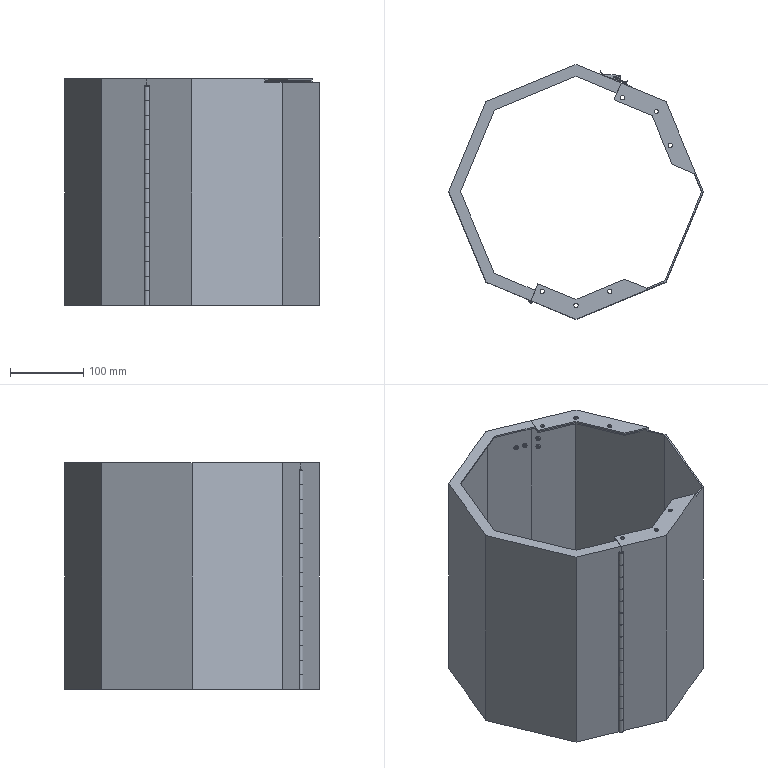Part | SolidWorks | features CompositeCurve 4 | 15 solids | 494 faces | box 348.53 x 348.53 x 310 mm | volume 714229 mm3 | cylinder 229 | plane 229 | cone 20 | torus 16 | commonest cylinder face diameters 6 x52 6.5 x45 3.5 x36 3 x26 2 x22 2.5 x16